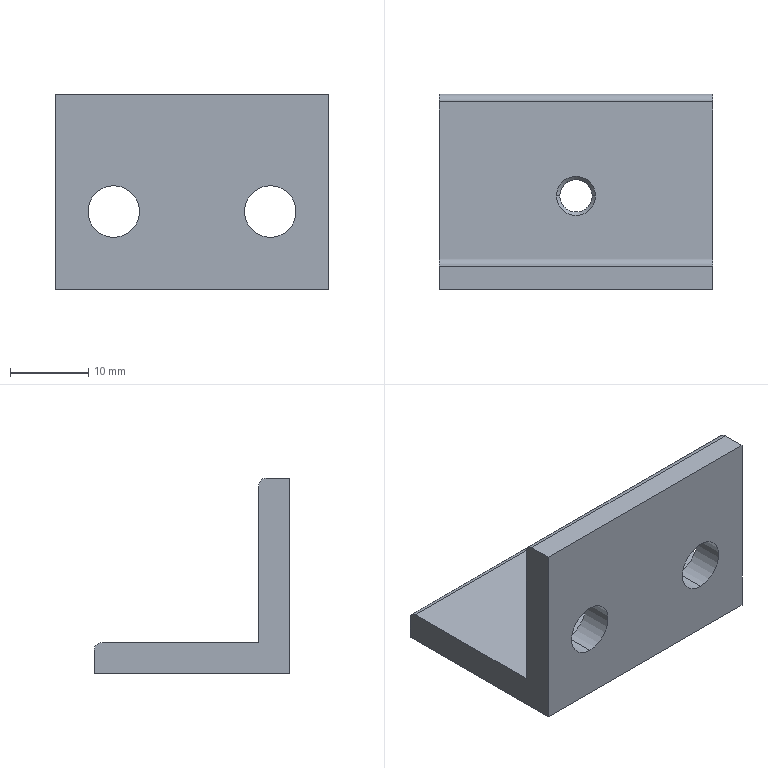Part | STEP file | hcba6_2_14a_Default | 1 solid | 20 faces | box 35 x 25 x 25 mm | volume 6095 mm3 | cylinder 8 | plane 8 | cone 4 | commonest cylinder face diameters 6.6 x4 2 x2 4.134 x2